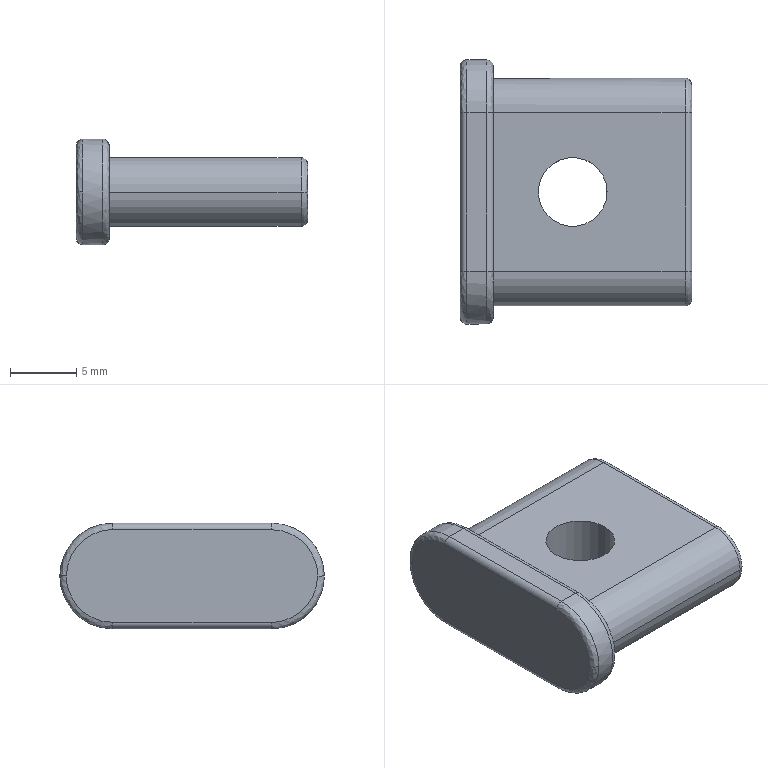Part | SolidWorks | features BaseBody 1 | 1 solid | 31 faces | box 17.5 x 20 x 8 mm | volume 1504 mm3 | cylinder 14 | spline 10 | plane 7 | commonest cylinder face diameters 1 x6 5.2 x5 8 x3
STEP:
#1=CARTESIAN_POINT('',(-91538.135,-120061.55,4564.099));
#2=VERTEX_POINT('',#1);
#3=CARTESIAN_POINT('',(-91538.135,-120058.95,4566.699));
#4=VERTEX_POINT('',#3);
#5=CARTESIAN_POINT('',(-91538.135,-120058.95,4564.099));
#6=DIRECTION('',(-1.,0.000000008,0.));
#7=DIRECTION('',(-0.000000008,-1.,0.));
#8=AXIS2_PLACEMENT_3D('',#5,#6,#7);
#9=CIRCLE('',#8,2.6);
#10=EDGE_CURVE('',#2,#4,#9,.T.);
#11=ORIENTED_EDGE('',*,*,#10,.F.);
#12=CARTESIAN_POINT('',(-91537.635,-120061.05,4564.099));
#13=VERTEX_POINT('',#12);
#14=CARTESIAN_POINT('',(-91538.135,-120061.05,4564.099));
#15=DIRECTION('',(0.,0.,1.));
#16=DIRECTION('',(-0.000000008,-1.,0.));
#17=AXIS2_PLACEMENT_3D('',#14,#15,#16);
#18=CIRCLE('',#17,0.5);
#19=EDGE_CURVE('',#2,#13,#18,.T.);
#20=ORIENTED_EDGE('',*,*,#19,.T.);
#21=CARTESIAN_POINT('',(-91537.635,-120058.95,4566.199));
#22=VERTEX_POINT('',#21);
#23=CARTESIAN_POINT('',(-91537.635,-120061.05,4564.099));
#24=CARTESIAN_POINT('',(-91537.635,-120061.05,4565.329));
#25=CARTESIAN_POINT('',(-91537.635,-120060.18,4566.199));
#26=CARTESIAN_POINT('',(-91537.635,-120058.95,4566.199));
#27=(BOUNDED_CURVE()B_SPLINE_CURVE(3,(#23,#24,#25,#26),.UNSPECIFIED.,.F.,.T.)B_SPLINE_CURVE_WITH_KNOTS((4,4),(0.,1.),.UNSPECIFIED.)CURVE()GEOMETRIC_REPRESENTATION_ITEM()RATIONAL_B_SPLINE_CURVE((1.,0.8047,0.8047,1.))REPRESENTATION_ITEM(''));
#28=EDGE_CURVE('',#13,#22,#27,.T.);
#29=ORIENTED_EDGE('',*,*,#28,.T.);
#30=CARTESIAN_POINT('',(-91538.135,-120058.95,4566.199));
#31=DIRECTION('',(-0.000000008,-1.,0.));
#32=DIRECTION('',(0.,0.,1.));
#33=AXIS2_PLACEMENT_3D('',#30,#31,#32);
#34=CIRCLE('',#33,0.5);
#35=EDGE_CURVE('',#22,#4,#34,.T.);
#36=ORIENTED_EDGE('',*,*,#35,.T.);
#37=EDGE_LOOP('',(#11,#20,#29,#36));
#38=FACE_OUTER_BOUND('',#37,.T.);
#39=CARTESIAN_POINT('',(-91538.135,-120061.55,4564.099));
#40=CARTESIAN_POINT('',(-91538.135,-120061.55,4565.633));
#41=CARTESIAN_POINT('',(-91538.135,-120060.46,4566.713));
#42=CARTESIAN_POINT('',(-91538.135,-120058.925,4566.699));
#43=CARTESIAN_POINT('',(-91537.842,-120061.55,4564.099));
#44=CARTESIAN_POINT('',(-91537.842,-120061.55,4565.633));
#45=CARTESIAN_POINT('',(-91537.842,-120060.46,4566.713));
#46=CARTESIAN_POINT('',(-91537.842,-120058.925,4566.699));
#47=CARTESIAN_POINT('',(-91537.635,-120061.343,4564.099));
#48=CARTESIAN_POINT('',(-91537.635,-120061.343,4565.511));
#49=CARTESIAN_POINT('',(-91537.635,-120060.34,4566.505));
#50=CARTESIAN_POINT('',(-91537.635,-120058.927,4566.492));
#51=CARTESIAN_POINT('',(-91537.635,-120061.05,4564.099));
#52=CARTESIAN_POINT('',(-91537.635,-120061.05,4565.338));
#53=CARTESIAN_POINT('',(-91537.635,-120060.17,4566.211));
#54=CARTESIAN_POINT('',(-91537.635,-120058.93,4566.199));
#55=(BOUNDED_SURFACE()B_SPLINE_SURFACE(3,3,((#39,#40,#41,#42),(#43,#44,#45,#46),(#47,#48,#49,#50),(#51,#52,#53,#54)),.UNSPECIFIED.,.F.,.F.,.F.)B_SPLINE_SURFACE_WITH_KNOTS((4,4),(4,4),(0.,1.),(0.,1.),.UNSPECIFIED.)GEOMETRIC_REPRESENTATION_ITEM()RATIONAL_B_SPLINE_SURFACE(((1.,0.8025,0.8025,1.),(0.8047,0.6458,0.6458,0.8047),(0.8047,0.6458,0.6458,0.8047),(1.,0.8025,0.8025,1.)))REPRESENTATION_ITEM('')SURFACE());
#56=ADVANCED_FACE('',(#38),#55,.T.);
#57=CARTESIAN_POINT('',(-91555.135,-120058.95,4567.599));
#58=VERTEX_POINT('',#57);
#59=CARTESIAN_POINT('',(-91555.135,-120062.45,4564.099));
#60=VERTEX_POINT('',#59);
#61=CARTESIAN_POINT('',(-91555.135,-120058.95,4567.599));
#62=CARTESIAN_POINT('',(-91555.135,-120061.,4567.599));
#63=CARTESIAN_POINT('',(-91555.135,-120062.45,4566.149));
#64=CARTESIAN_POINT('',(-91555.135,-120062.45,4564.099));
#65=(BOUNDED_CURVE()B_SPLINE_CURVE(3,(#61,#62,#63,#64),.UNSPECIFIED.,.F.,.T.)B_SPLINE_CURVE_WITH_KNOTS((4,4),(0.,1.),.UNSPECIFIED.)CURVE()GEOMETRIC_REPRESENTATION_ITEM()RATIONAL_B_SPLINE_CURVE((1.,0.8047,0.8047,1.))REPRESENTATION_ITEM(''));
#66=EDGE_CURVE('',#58,#60,#65,.T.);
#67=ORIENTED_EDGE('',*,*,#66,.T.);
#68=CARTESIAN_POINT('',(-91554.635,-120062.95,4564.099));
#69=VERTEX_POINT('',#68);
#70=CARTESIAN_POINT('',(-91554.635,-120062.45,4564.099));
#71=DIRECTION('',(0.,0.,1.));
#72=DIRECTION('',(-0.000000008,-1.,0.));
#73=AXIS2_PLACEMENT_3D('',#70,#71,#72);
#74=CIRCLE('',#73,0.5);
#75=EDGE_CURVE('',#60,#69,#74,.T.);
#76=ORIENTED_EDGE('',*,*,#75,.T.);
#77=CARTESIAN_POINT('',(-91554.635,-120058.95,4568.099));
#78=VERTEX_POINT('',#77);
#79=CARTESIAN_POINT('',(-91554.635,-120058.95,4564.099));
#80=DIRECTION('',(1.,-0.000000008,0.));
#81=DIRECTION('',(0.000000008,1.,0.));
#82=AXIS2_PLACEMENT_3D('',#79,#80,#81);
#83=CIRCLE('',#82,4.);
#84=EDGE_CURVE('',#78,#69,#83,.T.);
#85=ORIENTED_EDGE('',*,*,#84,.F.);
#86=CARTESIAN_POINT('',(-91554.635,-120058.95,4567.599));
#87=DIRECTION('',(0.000000008,1.,0.));
#88=DIRECTION('',(-1.,0.000000008,0.));
#89=AXIS2_PLACEMENT_3D('',#86,#87,#88);
#90=CIRCLE('',#89,0.5);
#91=EDGE_CURVE('',#58,#78,#90,.T.);
#92=ORIENTED_EDGE('',*,*,#91,.F.);
#93=EDGE_LOOP('',(#67,#76,#85,#92));
#94=FACE_OUTER_BOUND('',#93,.T.);
#95=CARTESIAN_POINT('',(-91555.135,-120062.45,4564.099));
#96=CARTESIAN_POINT('',(-91555.135,-120062.45,4566.149));
#97=CARTESIAN_POINT('',(-91555.135,-120061.,4567.599));
#98=CARTESIAN_POINT('',(-91555.135,-120058.95,4567.599));
#99=CARTESIAN_POINT('',(-91555.135,-120062.743,4564.099));
#100=CARTESIAN_POINT('',(-91555.135,-120062.743,4566.321));
#101=CARTESIAN_POINT('',(-91555.135,-120061.172,4567.892));
#102=CARTESIAN_POINT('',(-91555.135,-120058.95,4567.892));
#103=CARTESIAN_POINT('',(-91554.928,-120062.95,4564.099));
#104=CARTESIAN_POINT('',(-91554.928,-120062.95,4566.442));
#105=CARTESIAN_POINT('',(-91554.928,-120061.293,4568.099));
#106=CARTESIAN_POINT('',(-91554.928,-120058.95,4568.099));
#107=CARTESIAN_POINT('',(-91554.635,-120062.95,4564.099));
#108=CARTESIAN_POINT('',(-91554.635,-120062.95,4566.442));
#109=CARTESIAN_POINT('',(-91554.635,-120061.293,4568.099));
#110=CARTESIAN_POINT('',(-91554.635,-120058.95,4568.099));
#111=(BOUNDED_SURFACE()B_SPLINE_SURFACE(3,3,((#95,#96,#97,#98),(#99,#100,#101,#102),(#103,#104,#105,#106),(#107,#108,#109,#110)),.UNSPECIFIED.,.F.,.F.,.T.)B_SPLINE_SURFACE_WITH_KNOTS((4,4),(4,4),(0.,1.),(0.,1.),.UNSPECIFIED.)GEOMETRIC_REPRESENTATION_ITEM()RATIONAL_B_SPLINE_SURFACE(((1.,0.8047,0.8047,1.),(0.8047,0.6476,0.6476,0.8047),(0.8047,0.6476,0.6476,0.8047),(1.,0.8047,0.8047,1.)))REPRESENTATION_ITEM('')SURFACE());
#112=ADVANCED_FACE('',(#94),#111,.T.);
#113=CARTESIAN_POINT('',(-91538.135,-120058.95,4561.499));
#114=VERTEX_POINT('',#113);
#115=CARTESIAN_POINT('',(-91538.135,-120058.95,4564.099));
#116=DIRECTION('',(-1.,0.000000008,0.));
#117=DIRECTION('',(-0.000000008,-1.,0.));
#118=AXIS2_PLACEMENT_3D('',#115,#116,#117);
#119=CIRCLE('',#118,2.6);
#120=EDGE_CURVE('',#114,#2,#119,.T.);
#121=ORIENTED_EDGE('',*,*,#120,.T.);
#122=CARTESIAN_POINT('',(-91552.635,-120061.55,4564.099));
#123=VERTEX_POINT('',#122);
#124=CARTESIAN_POINT('',(-91519.666,-120061.55,4564.099));
#125=DIRECTION('',(-1.,0.000000008,0.));
#126=VECTOR('',#125,1000.);
#127=LINE('',#124,#126);
#128=EDGE_CURVE('',#2,#123,#127,.T.);
#129=ORIENTED_EDGE('',*,*,#128,.T.);
#130=CARTESIAN_POINT('',(-91552.635,-120058.95,4561.499));
#131=VERTEX_POINT('',#130);
#132=CARTESIAN_POINT('',(-91552.635,-120058.95,4564.099));
#133=DIRECTION('',(1.,-0.000000008,0.));
#134=DIRECTION('',(-0.000000008,-1.,0.));
#135=AXIS2_PLACEMENT_3D('',#132,#133,#134);
#136=CIRCLE('',#135,2.6);
#137=EDGE_CURVE('',#123,#131,#136,.T.);
#138=ORIENTED_EDGE('',*,*,#137,.T.);
#139=CARTESIAN_POINT('',(-91537.635,-120058.95,4561.499));
#140=DIRECTION('',(-1.,0.,0.));
#141=VECTOR('',#140,1000.);
#142=LINE('',#139,#141);
#143=EDGE_CURVE('',#114,#131,#142,.T.);
#144=ORIENTED_EDGE('',*,*,#143,.F.);
#145=EDGE_LOOP('',(#121,#129,#138,#144));
#146=FACE_OUTER_BOUND('',#145,.T.);
#147=CARTESIAN_POINT('',(-91519.666,-120058.95,4564.099));
#148=DIRECTION('',(-1.,0.000000008,0.));
#149=DIRECTION('',(-0.000000008,-1.,0.));
#150=AXIS2_PLACEMENT_3D('',#147,#148,#149);
#151=CYLINDRICAL_SURFACE('',#150,2.6);
#152=ADVANCED_FACE('',(#146),#151,.T.);
#153=CARTESIAN_POINT('',(-91544.035,-120052.95,4566.699));
#154=VERTEX_POINT('',#153);
#155=CARTESIAN_POINT('',(-91549.235,-120052.95,4566.699));
#156=VERTEX_POINT('',#155);
#157=CARTESIAN_POINT('',(-91546.635,-120052.95,4566.699));
#158=DIRECTION('',(0.,0.,-1.));
#159=DIRECTION('',(-1.,0.,0.));
#160=AXIS2_PLACEMENT_3D('',#157,#158,#159);
#161=CIRCLE('',#160,2.6);
#162=EDGE_CURVE('',#154,#156,#161,.T.);
#163=ORIENTED_EDGE('',*,*,#162,.F.);
#164=CARTESIAN_POINT('',(-91544.035,-120052.95,4561.499));
#165=VERTEX_POINT('',#164);
#166=CARTESIAN_POINT('',(-91544.035,-120052.95,4571.499));
#167=DIRECTION('',(0.,0.,-1.));
#168=VECTOR('',#167,1000.);
#169=LINE('',#166,#168);
#170=EDGE_CURVE('',#154,#165,#169,.T.);
#171=ORIENTED_EDGE('',*,*,#170,.T.);
#172=CARTESIAN_POINT('',(-91549.235,-120052.95,4561.499));
#173=VERTEX_POINT('',#172);
#174=CARTESIAN_POINT('',(-91546.635,-120052.95,4561.499));
#175=DIRECTION('',(0.,0.,1.));
#176=DIRECTION('',(-1.,0.,0.));
#177=AXIS2_PLACEMENT_3D('',#174,#175,#176);
#178=CIRCLE('',#177,2.6);
#179=EDGE_CURVE('',#173,#165,#178,.T.);
#180=ORIENTED_EDGE('',*,*,#179,.F.);
#181=CARTESIAN_POINT('',(-91549.235,-120052.95,4571.499));
#182=DIRECTION('',(0.,0.,-1.));
#183=VECTOR('',#182,1000.);
#184=LINE('',#181,#183);
#185=EDGE_CURVE('',#156,#173,#184,.T.);
#186=ORIENTED_EDGE('',*,*,#185,.F.);
#187=EDGE_LOOP('',(#163,#171,#180,#186));
#188=FACE_OUTER_BOUND('',#187,.T.);
#189=CARTESIAN_POINT('',(-91546.635,-120052.95,4571.499));
#190=DIRECTION('',(0.,0.,-1.));
#191=DIRECTION('',(-1.,0.,0.));
#192=AXIS2_PLACEMENT_3D('',#189,#190,#191);
#193=CYLINDRICAL_SURFACE('',#192,2.6);
#194=ADVANCED_FACE('',(#188),#193,.F.);
#195=CARTESIAN_POINT('',(-91554.635,-120046.95,4560.099));
#196=VERTEX_POINT('',#195);
#197=CARTESIAN_POINT('',(-91554.635,-120042.95,4564.099));
#198=VERTEX_POINT('',#197);
#199=CARTESIAN_POINT('',(-91554.635,-120046.95,4564.099));
#200=DIRECTION('',(1.,-0.000000008,0.));
#201=DIRECTION('',(0.000000008,1.,0.));
#202=AXIS2_PLACEMENT_3D('',#199,#200,#201);
#203=CIRCLE('',#202,4.);
#204=EDGE_CURVE('',#196,#198,#203,.T.);
#205=ORIENTED_EDGE('',*,*,#204,.T.);
#206=CARTESIAN_POINT('',(-91553.135,-120042.95,4564.099));
#207=VERTEX_POINT('',#206);
#208=CARTESIAN_POINT('',(-91576.676,-120042.95,4564.099));
#209=DIRECTION('',(1.,-0.000000008,0.));
#210=VECTOR('',#209,1000.);
#211=LINE('',#208,#210);
#212=EDGE_CURVE('',#198,#207,#211,.T.);
#213=ORIENTED_EDGE('',*,*,#212,.T.);
#214=CARTESIAN_POINT('',(-91553.135,-120046.95,4560.099));
#215=VERTEX_POINT('',#214);
#216=CARTESIAN_POINT('',(-91553.135,-120046.95,4564.099));
#217=DIRECTION('',(1.,-0.000000008,0.));
#218=DIRECTION('',(0.000000008,1.,0.));
#219=AXIS2_PLACEMENT_3D('',#216,#217,#218);
#220=CIRCLE('',#219,4.);
#221=EDGE_CURVE('',#215,#207,#220,.T.);
#222=ORIENTED_EDGE('',*,*,#221,.F.);
#223=CARTESIAN_POINT('',(-91576.676,-120046.95,4560.099));
#224=DIRECTION('',(-1.,0.000000008,0.));
#225=VECTOR('',#224,1000.);
#226=LINE('',#223,#225);
#227=EDGE_CURVE('',#215,#196,#226,.T.);
#228=ORIENTED_EDGE('',*,*,#227,.T.);
#229=EDGE_LOOP('',(#205,#213,#222,#228));
#230=FACE_OUTER_BOUND('',#229,.T.);
#231=CARTESIAN_POINT('',(-91576.676,-120046.95,4564.099));
#232=DIRECTION('',(1.,-0.000000008,0.));
#233=DIRECTION('',(0.000000008,1.,0.));
#234=AXIS2_PLACEMENT_3D('',#231,#232,#233);
#235=CYLINDRICAL_SURFACE('',#234,4.);
#236=ADVANCED_FACE('',(#230),#235,.T.);
#237=ORIENTED_EDGE('',*,*,#143,.T.);
#238=CARTESIAN_POINT('',(-91552.635,-120046.95,4561.499));
#239=VERTEX_POINT('',#238);
#240=CARTESIAN_POINT('',(-91552.635,-120048.95,4561.499));
#241=DIRECTION('',(0.,1.,0.));
#242=VECTOR('',#241,1000.);
#243=LINE('',#240,#242);
#244=EDGE_CURVE('',#131,#239,#243,.T.);
#245=ORIENTED_EDGE('',*,*,#244,.T.);
#246=CARTESIAN_POINT('',(-91538.135,-120046.95,4561.499));
#247=VERTEX_POINT('',#246);
#248=CARTESIAN_POINT('',(-91537.635,-120046.95,4561.499));
#249=DIRECTION('',(1.,0.,0.));
#250=VECTOR('',#249,1000.);
#251=LINE('',#248,#250);
#252=EDGE_CURVE('',#239,#247,#251,.T.);
#253=ORIENTED_EDGE('',*,*,#252,.T.);
#254=CARTESIAN_POINT('',(-91538.135,-120048.95,4561.499));
#255=DIRECTION('',(0.,-1.,0.));
#256=VECTOR('',#255,1000.);
#257=LINE('',#254,#256);
#258=EDGE_CURVE('',#247,#114,#257,.T.);
#259=ORIENTED_EDGE('',*,*,#258,.T.);
#260=EDGE_LOOP('',(#237,#245,#253,#259));
#261=FACE_OUTER_BOUND('',#260,.T.);
#262=ORIENTED_EDGE('',*,*,#179,.T.);
#263=CARTESIAN_POINT('',(-91546.635,-120052.95,4561.499));
#264=DIRECTION('',(0.,0.,1.));
#265=DIRECTION('',(-1.,0.,0.));
#266=AXIS2_PLACEMENT_3D('',#263,#264,#265);
#267=CIRCLE('',#266,2.6);
#268=EDGE_CURVE('',#165,#173,#267,.T.);
#269=ORIENTED_EDGE('',*,*,#268,.T.);
#270=EDGE_LOOP('',(#262,#269));
#271=FACE_BOUND('',#270,.T.);
#272=CARTESIAN_POINT('',(-91537.635,-120048.95,4561.499));
#273=DIRECTION('',(0.,0.,-1.));
#274=DIRECTION('',(-1.,0.,0.));
#275=AXIS2_PLACEMENT_3D('',#272,#273,#274);
#276=PLANE('',#275);
#277=ADVANCED_FACE('',(#261,#271),#276,.T.);
#278=CARTESIAN_POINT('',(-91552.635,-120058.95,4566.699));
#279=VERTEX_POINT('',#278);
#280=CARTESIAN_POINT('',(-91552.635,-120058.95,4564.099));
#281=DIRECTION('',(1.,-0.000000008,0.));
#282=DIRECTION('',(-0.000000008,-1.,0.));
#283=AXIS2_PLACEMENT_3D('',#280,#281,#282);
#284=CIRCLE('',#283,2.6);
#285=EDGE_CURVE('',#279,#123,#284,.T.);
#286=ORIENTED_EDGE('',*,*,#285,.F.);
#287=CARTESIAN_POINT('',(-91552.635,-120046.95,4566.699));
#288=VERTEX_POINT('',#287);
#289=CARTESIAN_POINT('',(-91552.635,-120056.95,4566.699));
#290=DIRECTION('',(-0.000000008,-1.,0.));
#291=VECTOR('',#290,1000.);
#292=LINE('',#289,#291);
#293=EDGE_CURVE('',#288,#279,#292,.T.);
#294=ORIENTED_EDGE('',*,*,#293,.F.);
#295=CARTESIAN_POINT('',(-91552.635,-120046.95,4564.099));
#296=DIRECTION('',(1.,-0.000000008,0.));
#297=DIRECTION('',(-0.000000008,-1.,0.));
#298=AXIS2_PLACEMENT_3D('',#295,#296,#297);
#299=CIRCLE('',#298,2.6);
#300=EDGE_CURVE('',#239,#288,#299,.T.);
#301=ORIENTED_EDGE('',*,*,#300,.F.);
#302=ORIENTED_EDGE('',*,*,#244,.F.);
#303=ORIENTED_EDGE('',*,*,#137,.F.);
#304=EDGE_LOOP('',(#286,#294,#301,#302,#303));
#305=FACE_BOUND('',#304,.T.);
#306=CARTESIAN_POINT('',(-91552.635,-120058.95,4567.599));
#307=VERTEX_POINT('',#306);
#308=CARTESIAN_POINT('',(-91552.635,-120046.95,4567.599));
#309=VERTEX_POINT('',#308);
#310=CARTESIAN_POINT('',(-91552.635,-120056.95,4567.599));
#311=DIRECTION('',(0.000000008,1.,0.));
#312=VECTOR('',#311,1000.);
#313=LINE('',#310,#312);
#314=EDGE_CURVE('',#307,#309,#313,.T.);
#315=ORIENTED_EDGE('',*,*,#314,.F.);
#316=CARTESIAN_POINT('',(-91552.635,-120058.95,4560.599));
#317=VERTEX_POINT('',#316);
#318=CARTESIAN_POINT('',(-91552.635,-120058.95,4560.599));
#319=CARTESIAN_POINT('',(-91552.635,-120065.95,4560.599));
#320=CARTESIAN_POINT('',(-91552.635,-120065.95,4567.599));
#321=CARTESIAN_POINT('',(-91552.635,-120058.95,4567.599));
#322=(BOUNDED_CURVE()B_SPLINE_CURVE(3,(#318,#319,#320,#321),.UNSPECIFIED.,.F.,.F.)B_SPLINE_CURVE_WITH_KNOTS((4,4),(0.,1.),.UNSPECIFIED.)CURVE()GEOMETRIC_REPRESENTATION_ITEM()RATIONAL_B_SPLINE_CURVE((1.,0.3333,0.3333,1.))REPRESENTATION_ITEM(''));
#323=EDGE_CURVE('',#317,#307,#322,.T.);
#324=ORIENTED_EDGE('',*,*,#323,.F.);
#325=CARTESIAN_POINT('',(-91552.635,-120046.95,4560.599));
#326=VERTEX_POINT('',#325);
#327=CARTESIAN_POINT('',(-91552.635,-120056.95,4560.599));
#328=DIRECTION('',(-0.000000008,-1.,0.));
#329=VECTOR('',#328,1000.);
#330=LINE('',#327,#329);
#331=EDGE_CURVE('',#326,#317,#330,.T.);
#332=ORIENTED_EDGE('',*,*,#331,.F.);
#333=CARTESIAN_POINT('',(-91552.635,-120046.95,4567.599));
#334=CARTESIAN_POINT('',(-91552.635,-120039.95,4567.599));
#335=CARTESIAN_POINT('',(-91552.635,-120039.95,4560.599));
#336=CARTESIAN_POINT('',(-91552.635,-120046.95,4560.599));
#337=(BOUNDED_CURVE()B_SPLINE_CURVE(3,(#333,#334,#335,#336),.UNSPECIFIED.,.F.,.F.)B_SPLINE_CURVE_WITH_KNOTS((4,4),(0.,1.),.UNSPECIFIED.)CURVE()GEOMETRIC_REPRESENTATION_ITEM()RATIONAL_B_SPLINE_CURVE((1.,0.3333,0.3333,1.))REPRESENTATION_ITEM(''));
#338=EDGE_CURVE('',#309,#326,#337,.T.);
#339=ORIENTED_EDGE('',*,*,#338,.F.);
#340=EDGE_LOOP('',(#315,#324,#332,#339));
#341=FACE_OUTER_BOUND('',#340,.T.);
#342=CARTESIAN_POINT('',(-91552.635,-120056.95,4564.099));
#343=DIRECTION('',(-1.,0.000000008,0.));
#344=DIRECTION('',(-0.000000008,-1.,0.));
#345=AXIS2_PLACEMENT_3D('',#342,#343,#344);
#346=PLANE('',#345);
#347=ADVANCED_FACE('',(#305,#341),#346,.F.);
#348=ORIENTED_EDGE('',*,*,#128,.F.);
#349=ORIENTED_EDGE('',*,*,#10,.T.);
#350=CARTESIAN_POINT('',(-91519.666,-120058.95,4566.699));
#351=DIRECTION('',(-1.,0.000000008,0.));
#352=VECTOR('',#351,1000.);
#353=LINE('',#350,#352);
#354=EDGE_CURVE('',#4,#279,#353,.T.);
#355=ORIENTED_EDGE('',*,*,#354,.T.);
#356=ORIENTED_EDGE('',*,*,#285,.T.);
#357=EDGE_LOOP('',(#348,#349,#355,#356));
#358=FACE_OUTER_BOUND('',#357,.T.);
#359=CARTESIAN_POINT('',(-91519.666,-120058.95,4564.099));
#360=DIRECTION('',(-1.,0.000000008,0.));
#361=DIRECTION('',(-0.000000008,-1.,0.));
#362=AXIS2_PLACEMENT_3D('',#359,#360,#361);
#363=CYLINDRICAL_SURFACE('',#362,2.6);
#364=ADVANCED_FACE('',(#358),#363,.T.);
#365=CARTESIAN_POINT('',(-91537.635,-120058.95,4561.999));
#366=VERTEX_POINT('',#365);
#367=CARTESIAN_POINT('',(-91538.135,-120058.95,4561.999));
#368=DIRECTION('',(0.000000008,1.,0.));
#369=DIRECTION('',(-1.,0.000000008,0.));
#370=AXIS2_PLACEMENT_3D('',#367,#368,#369);
#371=CIRCLE('',#370,0.5);
#372=EDGE_CURVE('',#366,#114,#371,.T.);
#373=ORIENTED_EDGE('',*,*,#372,.T.);
#374=ORIENTED_EDGE('',*,*,#258,.F.);
#375=CARTESIAN_POINT('',(-91537.635,-120046.95,4561.999));
#376=VERTEX_POINT('',#375);
#377=CARTESIAN_POINT('',(-91538.135,-120046.95,4561.999));
#378=DIRECTION('',(0.000000008,1.,0.));
#379=DIRECTION('',(-1.,0.000000008,0.));
#380=AXIS2_PLACEMENT_3D('',#377,#378,#379);
#381=CIRCLE('',#380,0.5);
#382=EDGE_CURVE('',#376,#247,#381,.T.);
#383=ORIENTED_EDGE('',*,*,#382,.F.);
#384=CARTESIAN_POINT('',(-91537.635,-120048.95,4561.999));
#385=DIRECTION('',(-0.000000008,-1.,0.));
#386=VECTOR('',#385,1000.);
#387=LINE('',#384,#386);
#388=EDGE_CURVE('',#376,#366,#387,.T.);
#389=ORIENTED_EDGE('',*,*,#388,.T.);
#390=EDGE_LOOP('',(#373,#374,#383,#389));
#391=FACE_OUTER_BOUND('',#390,.T.);
#392=CARTESIAN_POINT('',(-91538.135,-120048.95,4561.999));
#393=DIRECTION('',(0.000000008,1.,0.));
#394=DIRECTION('',(-1.,0.000000008,0.));
#395=AXIS2_PLACEMENT_3D('',#392,#393,#394);
#396=CYLINDRICAL_SURFACE('',#395,0.5);
#397=ADVANCED_FACE('',(#391),#396,.T.);
#398=CARTESIAN_POINT('',(-91538.135,-120046.95,4566.699));
#399=VERTEX_POINT('',#398);
#400=CARTESIAN_POINT('',(-91519.666,-120046.95,4566.699));
#401=DIRECTION('',(1.,-0.000000008,0.));
#402=VECTOR('',#401,1000.);
#403=LINE('',#400,#402);
#404=EDGE_CURVE('',#288,#399,#403,.T.);
#405=ORIENTED_EDGE('',*,*,#404,.T.);
#406=CARTESIAN_POINT('',(-91538.135,-120044.35,4564.099));
#407=VERTEX_POINT('',#406);
#408=CARTESIAN_POINT('',(-91538.135,-120046.95,4564.099));
#409=DIRECTION('',(-1.,0.000000008,0.));
#410=DIRECTION('',(-0.000000008,-1.,0.));
#411=AXIS2_PLACEMENT_3D('',#408,#409,#410);
#412=CIRCLE('',#411,2.6);
#413=EDGE_CURVE('',#399,#407,#412,.T.);
#414=ORIENTED_EDGE('',*,*,#413,.T.);
#415=CARTESIAN_POINT('',(-91538.135,-120046.95,4564.099));
#416=DIRECTION('',(-1.,0.000000008,0.));
#417=DIRECTION('',(-0.000000008,-1.,0.));
#418=AXIS2_PLACEMENT_3D('',#415,#416,#417);
#419=CIRCLE('',#418,2.6);
#420=EDGE_CURVE('',#407,#247,#419,.T.);
#421=ORIENTED_EDGE('',*,*,#420,.T.);
#422=ORIENTED_EDGE('',*,*,#252,.F.);
#423=ORIENTED_EDGE('',*,*,#300,.T.);
#424=EDGE_LOOP('',(#405,#414,#421,#422,#423));
#425=FACE_OUTER_BOUND('',#424,.T.);
#426=CARTESIAN_POINT('',(-91519.666,-120046.95,4564.099));
#427=DIRECTION('',(-1.,0.000000008,0.));
#428=DIRECTION('',(-0.000000008,-1.,0.));
#429=AXIS2_PLACEMENT_3D('',#426,#427,#428);
#430=CYLINDRICAL_SURFACE('',#429,2.6);
#431=ADVANCED_FACE('',(#425),#430,.T.);
#432=ORIENTED_EDGE('',*,*,#170,.F.);
#433=CARTESIAN_POINT('',(-91546.635,-120052.95,4566.699));
#434=DIRECTION('',(0.,0.,-1.));
#435=DIRECTION('',(-1.,0.,0.));
#436=AXIS2_PLACEMENT_3D('',#433,#434,#435);
#437=CIRCLE('',#436,2.6);
#438=EDGE_CURVE('',#156,#154,#437,.T.);
#439=ORIENTED_EDGE('',*,*,#438,.F.);
#440=ORIENTED_EDGE('',*,*,#185,.T.);
#441=ORIENTED_EDGE('',*,*,#268,.F.);
#442=EDGE_LOOP('',(#432,#439,#440,#441));
#443=FACE_OUTER_BOUND('',#442,.T.);
#444=CARTESIAN_POINT('',(-91546.635,-120052.95,4571.499));
#445=DIRECTION('',(0.,0.,-1.));
#446=DIRECTION('',(-1.,0.,0.));
#447=AXIS2_PLACEMENT_3D('',#444,#445,#446);
#448=CYLINDRICAL_SURFACE('',#447,2.6);
#449=ADVANCED_FACE('',(#443),#448,.F.);
#450=ORIENTED_EDGE('',*,*,#404,.F.);
#451=ORIENTED_EDGE('',*,*,#293,.T.);
#452=ORIENTED_EDGE('',*,*,#354,.F.);
#453=CARTESIAN_POINT('',(-91538.135,-120056.95,4566.699));
#454=DIRECTION('',(0.,1.,0.));
#455=VECTOR('',#454,1000.);
#456=LINE('',#453,#455);
#457=EDGE_CURVE('',#4,#399,#456,.T.);
#458=ORIENTED_EDGE('',*,*,#457,.T.);
#459=EDGE_LOOP('',(#450,#451,#452,#458));
#460=FACE_OUTER_BOUND('',#459,.T.);
#461=ORIENTED_EDGE('',*,*,#438,.T.);
#462=ORIENTED_EDGE('',*,*,#162,.T.);
#463=EDGE_LOOP('',(#461,#462));
#464=FACE_BOUND('',#463,.T.);
#465=CARTESIAN_POINT('',(-91537.635,-120056.95,4566.699));
#466=DIRECTION('',(0.,0.,1.));
#467=DIRECTION('',(1.,0.,0.));
#468=AXIS2_PLACEMENT_3D('',#465,#466,#467);
#469=PLANE('',#468);
#470=ADVANCED_FACE('',(#460,#464),#469,.T.);
#471=ORIENTED_EDGE('',*,*,#221,.T.);
#472=CARTESIAN_POINT('',(-91553.135,-120046.95,4568.099));
#473=VERTEX_POINT('',#472);
#474=CARTESIAN_POINT('',(-91553.135,-120046.95,4564.099));
#475=DIRECTION('',(1.,-0.000000008,0.));
#476=DIRECTION('',(0.000000008,1.,0.));
#477=AXIS2_PLACEMENT_3D('',#474,#475,#476);
#478=CIRCLE('',#477,4.);
#479=EDGE_CURVE('',#207,#473,#478,.T.);
#480=ORIENTED_EDGE('',*,*,#479,.T.);
#481=CARTESIAN_POINT('',(-91553.135,-120046.95,4567.599));
#482=DIRECTION('',(0.000000008,1.,0.));
#483=DIRECTION('',(-1.,0.000000008,0.));
#484=AXIS2_PLACEMENT_3D('',#481,#482,#483);
#485=CIRCLE('',#484,0.5);
#486=EDGE_CURVE('',#473,#309,#485,.T.);
#487=ORIENTED_EDGE('',*,*,#486,.T.);
#488=ORIENTED_EDGE('',*,*,#338,.T.);
#489=CARTESIAN_POINT('',(-91553.135,-120046.95,4560.599));
#490=DIRECTION('',(0.000000008,1.,0.));
#491=DIRECTION('',(-1.,0.000000008,0.));
#492=AXIS2_PLACEMENT_3D('',#489,#490,#491);
#493=CIRCLE('',#492,0.5);
#494=EDGE_CURVE('',#326,#215,#493,.T.);
#495=ORIENTED_EDGE('',*,*,#494,.T.);
#496=EDGE_LOOP('',(#471,#480,#487,#488,#495));
#497=FACE_OUTER_BOUND('',#496,.T.);
#498=CARTESIAN_POINT('',(-91553.135,-120046.95,4568.099));
#499=CARTESIAN_POINT('',(-91553.135,-120038.95,4568.099));
#500=CARTESIAN_POINT('',(-91553.135,-120038.95,4560.099));
#501=CARTESIAN_POINT('',(-91553.135,-120046.95,4560.099));
#502=CARTESIAN_POINT('',(-91552.842,-120046.95,4568.099));
#503=CARTESIAN_POINT('',(-91552.842,-120038.95,4568.099));
#504=CARTESIAN_POINT('',(-91552.842,-120038.95,4560.099));
#505=CARTESIAN_POINT('',(-91552.842,-120046.95,4560.099));
#506=CARTESIAN_POINT('',(-91552.635,-120046.95,4567.892));
#507=CARTESIAN_POINT('',(-91552.635,-120039.364,4567.892));
#508=CARTESIAN_POINT('',(-91552.635,-120039.364,4560.306));
#509=CARTESIAN_POINT('',(-91552.635,-120046.95,4560.306));
#510=CARTESIAN_POINT('',(-91552.635,-120046.95,4567.599));
#511=CARTESIAN_POINT('',(-91552.635,-120039.95,4567.599));
#512=CARTESIAN_POINT('',(-91552.635,-120039.95,4560.599));
#513=CARTESIAN_POINT('',(-91552.635,-120046.95,4560.599));
#514=(BOUNDED_SURFACE()B_SPLINE_SURFACE(3,3,((#498,#499,#500,#501),(#502,#503,#504,#505),(#506,#507,#508,#509),(#510,#511,#512,#513)),.UNSPECIFIED.,.F.,.F.,.T.)B_SPLINE_SURFACE_WITH_KNOTS((4,4),(4,4),(0.,1.),(0.,1.),.UNSPECIFIED.)GEOMETRIC_REPRESENTATION_ITEM()RATIONAL_B_SPLINE_SURFACE(((1.,0.3333,0.3333,1.),(0.8047,0.2682,0.2682,0.8047),(0.8047,0.2682,0.2682,0.8047),(1.,0.3333,0.3333,1.)))REPRESENTATION_ITEM('')SURFACE());
#515=ADVANCED_FACE('',(#497),#514,.T.);
#516=CARTESIAN_POINT('',(-91553.135,-120058.95,4568.099));
#517=VERTEX_POINT('',#516);
#518=CARTESIAN_POINT('',(-91553.135,-120058.95,4567.599));
#519=DIRECTION('',(0.000000008,1.,0.));
#520=DIRECTION('',(1.,-0.000000008,0.));
#521=AXIS2_PLACEMENT_3D('',#518,#519,#520);
#522=CIRCLE('',#521,0.5);
#523=EDGE_CURVE('',#517,#307,#522,.T.);
#524=ORIENTED_EDGE('',*,*,#523,.T.);
#525=ORIENTED_EDGE('',*,*,#314,.T.);
#526=ORIENTED_EDGE('',*,*,#486,.F.);
#527=CARTESIAN_POINT('',(-91553.135,-120056.95,4568.099));
#528=DIRECTION('',(-0.000000008,-1.,0.));
#529=VECTOR('',#528,1000.);
#530=LINE('',#527,#529);
#531=EDGE_CURVE('',#473,#517,#530,.T.);
#532=ORIENTED_EDGE('',*,*,#531,.T.);
#533=EDGE_LOOP('',(#524,#525,#526,#532));
#534=FACE_OUTER_BOUND('',#533,.T.);
#535=CARTESIAN_POINT('',(-91553.135,-120056.95,4567.599));
#536=DIRECTION('',(-0.000000008,-1.,0.));
#537=DIRECTION('',(1.,-0.000000008,0.));
#538=AXIS2_PLACEMENT_3D('',#535,#536,#537);
#539=CYLINDRICAL_SURFACE('',#538,0.5);
#540=ADVANCED_FACE('',(#534),#539,.T.);
#541=CARTESIAN_POINT('',(-91553.135,-120058.95,4560.099));
#542=VERTEX_POINT('',#541);
#543=CARTESIAN_POINT('',(-91553.135,-120058.95,4560.599));
#544=DIRECTION('',(-0.000000008,-1.,0.));
#545=DIRECTION('',(-1.,0.000000008,0.));
#546=AXIS2_PLACEMENT_3D('',#543,#544,#545);
#547=CIRCLE('',#546,0.5);
#548=EDGE_CURVE('',#542,#317,#547,.T.);
#549=ORIENTED_EDGE('',*,*,#548,.T.);
#550=ORIENTED_EDGE('',*,*,#323,.T.);
#551=ORIENTED_EDGE('',*,*,#523,.F.);
#552=CARTESIAN_POINT('',(-91553.135,-120058.95,4564.099));
#553=DIRECTION('',(1.,-0.000000008,0.));
#554=DIRECTION('',(0.000000008,1.,0.));
#555=AXIS2_PLACEMENT_3D('',#552,#553,#554);
#556=CIRCLE('',#555,4.);
#557=EDGE_CURVE('',#517,#542,#556,.T.);
#558=ORIENTED_EDGE('',*,*,#557,.T.);
#559=EDGE_LOOP('',(#549,#550,#551,#558));
#560=FACE_OUTER_BOUND('',#559,.T.);
#561=CARTESIAN_POINT('',(-91553.135,-120058.95,4560.099));
#562=CARTESIAN_POINT('',(-91553.135,-120066.95,4560.099));
#563=CARTESIAN_POINT('',(-91553.135,-120066.95,4568.099));
#564=CARTESIAN_POINT('',(-91553.135,-120058.95,4568.099));
#565=CARTESIAN_POINT('',(-91552.842,-120058.95,4560.099));
#566=CARTESIAN_POINT('',(-91552.842,-120066.95,4560.099));
#567=CARTESIAN_POINT('',(-91552.842,-120066.95,4568.099));
#568=CARTESIAN_POINT('',(-91552.842,-120058.95,4568.099));
#569=CARTESIAN_POINT('',(-91552.635,-120058.95,4560.306));
#570=CARTESIAN_POINT('',(-91552.635,-120066.536,4560.306));
#571=CARTESIAN_POINT('',(-91552.635,-120066.536,4567.892));
#572=CARTESIAN_POINT('',(-91552.635,-120058.95,4567.892));
#573=CARTESIAN_POINT('',(-91552.635,-120058.95,4560.599));
#574=CARTESIAN_POINT('',(-91552.635,-120065.95,4560.599));
#575=CARTESIAN_POINT('',(-91552.635,-120065.95,4567.599));
#576=CARTESIAN_POINT('',(-91552.635,-120058.95,4567.599));
#577=(BOUNDED_SURFACE()B_SPLINE_SURFACE(3,3,((#561,#562,#563,#564),(#565,#566,#567,#568),(#569,#570,#571,#572),(#573,#574,#575,#576)),.UNSPECIFIED.,.F.,.F.,.F.)B_SPLINE_SURFACE_WITH_KNOTS((4,4),(4,4),(0.,1.),(0.,1.),.UNSPECIFIED.)GEOMETRIC_REPRESENTATION_ITEM()RATIONAL_B_SPLINE_SURFACE(((1.,0.3333,0.3333,1.),(0.8047,0.2682,0.2682,0.8047),(0.8047,0.2682,0.2682,0.8047),(1.,0.3333,0.3333,1.)))REPRESENTATION_ITEM('')SURFACE());
#578=ADVANCED_FACE('',(#560),#577,.T.);
#579=ORIENTED_EDGE('',*,*,#494,.F.);
#580=ORIENTED_EDGE('',*,*,#331,.T.);
#581=ORIENTED_EDGE('',*,*,#548,.F.);
#582=CARTESIAN_POINT('',(-91553.135,-120056.95,4560.099));
#583=DIRECTION('',(0.000000008,1.,0.));
#584=VECTOR('',#583,1000.);
#585=LINE('',#582,#584);
#586=EDGE_CURVE('',#542,#215,#585,.T.);
#587=ORIENTED_EDGE('',*,*,#586,.T.);
#588=EDGE_LOOP('',(#579,#580,#581,#587));
#589=FACE_OUTER_BOUND('',#588,.T.);
#590=CARTESIAN_POINT('',(-91553.135,-120056.95,4560.599));
#591=DIRECTION('',(0.000000008,1.,0.));
#592=DIRECTION('',(-1.,0.000000008,0.));
#593=AXIS2_PLACEMENT_3D('',#590,#591,#592);
#594=CYLINDRICAL_SURFACE('',#593,0.5);
#595=ADVANCED_FACE('',(#589),#594,.T.);
#596=ORIENTED_EDGE('',*,*,#19,.F.);
#597=ORIENTED_EDGE('',*,*,#120,.F.);
#598=ORIENTED_EDGE('',*,*,#372,.F.);
#599=CARTESIAN_POINT('',(-91537.635,-120058.95,4561.999));
#600=CARTESIAN_POINT('',(-91537.635,-120059.175,4561.999));
#601=CARTESIAN_POINT('',(-91537.635,-120059.4,4562.036));
#602=CARTESIAN_POINT('',(-91537.635,-120059.721,4562.142));
#603=CARTESIAN_POINT('',(-91537.635,-120059.825,4562.187));
#604=CARTESIAN_POINT('',(-91537.635,-120059.974,4562.265));
#605=CARTESIAN_POINT('',(-91537.635,-120060.048,4562.307));
#606=CARTESIAN_POINT('',(-91537.635,-120060.13,4562.361));
#607=CARTESIAN_POINT('',(-91537.635,-120060.17,4562.39));
#608=CARTESIAN_POINT('',(-91537.635,-120060.19,4562.404));
#609=CARTESIAN_POINT('',(-91537.635,-120060.199,4562.411));
#610=CARTESIAN_POINT('',(-91537.635,-120060.204,4562.415));
#611=CARTESIAN_POINT('',(-91537.635,-120060.206,4562.416));
#612=CARTESIAN_POINT('',(-91537.635,-120060.332,4562.511));
#613=CARTESIAN_POINT('',(-91537.635,-120060.445,4562.617));
#614=CARTESIAN_POINT('',(-91537.635,-120060.594,4562.789));
#615=CARTESIAN_POINT('',(-91537.635,-120060.641,4562.85));
#616=CARTESIAN_POINT('',(-91537.635,-120060.706,4562.945));
#617=CARTESIAN_POINT('',(-91537.635,-120060.737,4562.993));
#618=CARTESIAN_POINT('',(-91537.635,-120060.771,4563.052));
#619=CARTESIAN_POINT('',(-91537.635,-120060.787,4563.081));
#620=CARTESIAN_POINT('',(-91537.635,-120060.795,4563.096));
#621=CARTESIAN_POINT('',(-91537.635,-120060.798,4563.102));
#622=CARTESIAN_POINT('',(-91537.635,-120060.801,4563.107));
#623=CARTESIAN_POINT('',(-91537.635,-120060.803,4563.111));
#624=CARTESIAN_POINT('',(-91537.635,-120060.81,4563.125));
#625=CARTESIAN_POINT('',(-91537.635,-120060.858,4563.206));
#626=CARTESIAN_POINT('',(-91537.635,-120060.948,4563.447));
#627=CARTESIAN_POINT('',(-91537.635,-120060.98,4563.548));
#628=CARTESIAN_POINT('',(-91537.635,-120061.031,4563.792));
#629=CARTESIAN_POINT('',(-91537.635,-120061.05,4563.935));
#630=CARTESIAN_POINT('',(-91537.635,-120061.05,4564.099));
#631=B_SPLINE_CURVE_WITH_KNOTS('',3,(#599,#600,#601,#602,#603,#604,#605,#606,#607,#608,#609,#610,#611,#612,#613,#614,#615,#616,#617,#618,#619,#620,#621,#622,#623,#624,#625,#626,#627,#628,#629,#630),.UNSPECIFIED.,.F.,.F.,(4,2,2,1,1,1,1,2,2,2,2,1,1,1,1,2,2,2,2,4),(0.,0.25,0.375,0.4375,0.4688,0.4844,0.4922,0.4961,0.5,0.625,0.6875,0.7188,0.7344,0.7422,0.7461,0.748,0.75,0.875,0.9375,1.),.UNSPECIFIED.);
#632=EDGE_CURVE('',#366,#13,#631,.T.);
#633=ORIENTED_EDGE('',*,*,#632,.T.);
#634=EDGE_LOOP('',(#596,#597,#598,#633));
#635=FACE_OUTER_BOUND('',#634,.T.);
#636=CARTESIAN_POINT('',(-91538.135,-120058.95,4561.499));
#637=CARTESIAN_POINT('',(-91538.135,-120060.473,4561.499));
#638=CARTESIAN_POINT('',(-91538.135,-120061.55,4562.576));
#639=CARTESIAN_POINT('',(-91538.135,-120061.55,4564.099));
#640=CARTESIAN_POINT('',(-91537.84,-120058.95,4561.499));
#641=CARTESIAN_POINT('',(-91537.84,-120060.473,4561.499));
#642=CARTESIAN_POINT('',(-91537.84,-120061.55,4562.576));
#643=CARTESIAN_POINT('',(-91537.84,-120061.55,4564.099));
#644=CARTESIAN_POINT('',(-91537.632,-120058.95,4561.709));
#645=CARTESIAN_POINT('',(-91537.632,-120060.35,4561.709));
#646=CARTESIAN_POINT('',(-91537.632,-120061.34,4562.699));
#647=CARTESIAN_POINT('',(-91537.632,-120061.34,4564.099));
#648=CARTESIAN_POINT('',(-91537.635,-120058.95,4562.004));
#649=CARTESIAN_POINT('',(-91537.635,-120060.177,4562.004));
#650=CARTESIAN_POINT('',(-91537.635,-120061.045,4562.872));
#651=CARTESIAN_POINT('',(-91537.635,-120061.045,4564.099));
#652=(BOUNDED_SURFACE()B_SPLINE_SURFACE(3,3,((#636,#637,#638,#639),(#640,#641,#642,#643),(#644,#645,#646,#647),(#648,#649,#650,#651)),.UNSPECIFIED.,.F.,.F.,.T.)B_SPLINE_SURFACE_WITH_KNOTS((4,4),(4,4),(0.,1.),(0.,1.),.UNSPECIFIED.)GEOMETRIC_REPRESENTATION_ITEM()RATIONAL_B_SPLINE_SURFACE(((1.,0.8047,0.8047,1.),(0.8025,0.6458,0.6458,0.8025),(0.8025,0.6458,0.6458,0.8025),(1.,0.8047,0.8047,1.)))REPRESENTATION_ITEM('')SURFACE());
#653=ADVANCED_FACE('',(#635),#652,.T.);
#654=CARTESIAN_POINT('',(-91537.635,-120044.85,4564.099));
#655=VERTEX_POINT('',#654);
#656=CARTESIAN_POINT('',(-91537.635,-120044.85,4564.099));
#657=CARTESIAN_POINT('',(-91537.635,-120044.85,4562.869));
#658=CARTESIAN_POINT('',(-91537.635,-120045.72,4561.999));
#659=CARTESIAN_POINT('',(-91537.635,-120046.95,4561.999));
#660=(BOUNDED_CURVE()B_SPLINE_CURVE(3,(#656,#657,#658,#659),.UNSPECIFIED.,.F.,.F.)B_SPLINE_CURVE_WITH_KNOTS((4,4),(0.,1.),.UNSPECIFIED.)CURVE()GEOMETRIC_REPRESENTATION_ITEM()RATIONAL_B_SPLINE_CURVE((1.,0.8047,0.8047,1.))REPRESENTATION_ITEM(''));
#661=EDGE_CURVE('',#655,#376,#660,.T.);
#662=ORIENTED_EDGE('',*,*,#661,.F.);
#663=CARTESIAN_POINT('',(-91537.635,-120046.95,4566.199));
#664=VERTEX_POINT('',#663);
#665=CARTESIAN_POINT('',(-91537.635,-120046.95,4566.199));
#666=CARTESIAN_POINT('',(-91537.635,-120045.72,4566.199));
#667=CARTESIAN_POINT('',(-91537.635,-120044.85,4565.329));
#668=CARTESIAN_POINT('',(-91537.635,-120044.85,4564.099));
#669=(BOUNDED_CURVE()B_SPLINE_CURVE(3,(#665,#666,#667,#668),.UNSPECIFIED.,.F.,.F.)B_SPLINE_CURVE_WITH_KNOTS((4,4),(0.,1.),.UNSPECIFIED.)CURVE()GEOMETRIC_REPRESENTATION_ITEM()RATIONAL_B_SPLINE_CURVE((1.,0.8047,0.8047,1.))REPRESENTATION_ITEM(''));
#670=EDGE_CURVE('',#664,#655,#669,.T.);
#671=ORIENTED_EDGE('',*,*,#670,.F.);
#672=CARTESIAN_POINT('',(-91537.635,-120056.95,4566.199));
#673=DIRECTION('',(0.000000008,1.,0.));
#674=VECTOR('',#673,1000.);
#675=LINE('',#672,#674);
#676=EDGE_CURVE('',#22,#664,#675,.T.);
#677=ORIENTED_EDGE('',*,*,#676,.F.);
#678=ORIENTED_EDGE('',*,*,#28,.F.);
#679=ORIENTED_EDGE('',*,*,#632,.F.);
#680=ORIENTED_EDGE('',*,*,#388,.F.);
#681=EDGE_LOOP('',(#662,#671,#677,#678,#679,#680));
#682=FACE_OUTER_BOUND('',#681,.T.);
#683=CARTESIAN_POINT('',(-91537.635,-120056.95,4564.099));
#684=DIRECTION('',(-1.,0.000000008,0.));
#685=DIRECTION('',(-0.000000008,-1.,0.));
#686=AXIS2_PLACEMENT_3D('',#683,#684,#685);
#687=PLANE('',#686);
#688=ADVANCED_FACE('',(#682),#687,.F.);
#689=CARTESIAN_POINT('',(-91538.135,-120044.85,4564.099));
#690=DIRECTION('',(0.,0.,1.));
#691=DIRECTION('',(1.,0.,0.));
#692=AXIS2_PLACEMENT_3D('',#689,#690,#691);
#693=CIRCLE('',#692,0.5);
#694=EDGE_CURVE('',#655,#407,#693,.T.);
#695=ORIENTED_EDGE('',*,*,#694,.T.);
#696=ORIENTED_EDGE('',*,*,#413,.F.);
#697=CARTESIAN_POINT('',(-91538.135,-120046.95,4566.199));
#698=DIRECTION('',(0.000000008,1.,0.));
#699=DIRECTION('',(1.,-0.000000008,0.));
#700=AXIS2_PLACEMENT_3D('',#697,#698,#699);
#701=CIRCLE('',#700,0.5);
#702=EDGE_CURVE('',#399,#664,#701,.T.);
#703=ORIENTED_EDGE('',*,*,#702,.T.);
#704=ORIENTED_EDGE('',*,*,#670,.T.);
#705=EDGE_LOOP('',(#695,#696,#703,#704));
#706=FACE_OUTER_BOUND('',#705,.T.);
#707=CARTESIAN_POINT('',(-91538.135,-120046.95,4566.699));
#708=CARTESIAN_POINT('',(-91538.135,-120045.427,4566.699));
#709=CARTESIAN_POINT('',(-91538.135,-120044.35,4565.622));
#710=CARTESIAN_POINT('',(-91538.135,-120044.35,4564.099));
#711=CARTESIAN_POINT('',(-91537.842,-120046.95,4566.699));
#712=CARTESIAN_POINT('',(-91537.842,-120045.427,4566.699));
#713=CARTESIAN_POINT('',(-91537.842,-120044.35,4565.622));
#714=CARTESIAN_POINT('',(-91537.842,-120044.35,4564.099));
#715=CARTESIAN_POINT('',(-91537.635,-120046.95,4566.492));
#716=CARTESIAN_POINT('',(-91537.635,-120045.548,4566.492));
#717=CARTESIAN_POINT('',(-91537.635,-120044.557,4565.501));
#718=CARTESIAN_POINT('',(-91537.635,-120044.557,4564.099));
#719=CARTESIAN_POINT('',(-91537.635,-120046.95,4566.199));
#720=CARTESIAN_POINT('',(-91537.635,-120045.72,4566.199));
#721=CARTESIAN_POINT('',(-91537.635,-120044.85,4565.329));
#722=CARTESIAN_POINT('',(-91537.635,-120044.85,4564.099));
#723=(BOUNDED_SURFACE()B_SPLINE_SURFACE(3,3,((#707,#708,#709,#710),(#711,#712,#713,#714),(#715,#716,#717,#718),(#719,#720,#721,#722)),.UNSPECIFIED.,.F.,.F.,.F.)B_SPLINE_SURFACE_WITH_KNOTS((4,4),(4,4),(0.,1.),(0.,1.),.UNSPECIFIED.)GEOMETRIC_REPRESENTATION_ITEM()RATIONAL_B_SPLINE_SURFACE(((1.,0.8047,0.8047,1.),(0.8047,0.6476,0.6476,0.8047),(0.8047,0.6476,0.6476,0.8047),(1.,0.8047,0.8047,1.)))REPRESENTATION_ITEM('')SURFACE());
#724=ADVANCED_FACE('',(#706),#723,.T.);
#725=ORIENTED_EDGE('',*,*,#420,.F.);
#726=ORIENTED_EDGE('',*,*,#694,.F.);
#727=ORIENTED_EDGE('',*,*,#661,.T.);
#728=ORIENTED_EDGE('',*,*,#382,.T.);
#729=EDGE_LOOP('',(#725,#726,#727,#728));
#730=FACE_OUTER_BOUND('',#729,.T.);
#731=CARTESIAN_POINT('',(-91538.135,-120044.35,4564.099));
#732=CARTESIAN_POINT('',(-91538.135,-120044.35,4562.576));
#733=CARTESIAN_POINT('',(-91538.135,-120045.427,4561.499));
#734=CARTESIAN_POINT('',(-91538.135,-120046.95,4561.499));
#735=CARTESIAN_POINT('',(-91537.842,-120044.35,4564.099));
#736=CARTESIAN_POINT('',(-91537.842,-120044.35,4562.576));
#737=CARTESIAN_POINT('',(-91537.842,-120045.427,4561.499));
#738=CARTESIAN_POINT('',(-91537.842,-120046.95,4561.499));
#739=CARTESIAN_POINT('',(-91537.635,-120044.557,4564.099));
#740=CARTESIAN_POINT('',(-91537.635,-120044.557,4562.697));
#741=CARTESIAN_POINT('',(-91537.635,-120045.548,4561.706));
#742=CARTESIAN_POINT('',(-91537.635,-120046.95,4561.706));
#743=CARTESIAN_POINT('',(-91537.635,-120044.85,4564.099));
#744=CARTESIAN_POINT('',(-91537.635,-120044.85,4562.869));
#745=CARTESIAN_POINT('',(-91537.635,-120045.72,4561.999));
#746=CARTESIAN_POINT('',(-91537.635,-120046.95,4561.999));
#747=(BOUNDED_SURFACE()B_SPLINE_SURFACE(3,3,((#731,#732,#733,#734),(#735,#736,#737,#738),(#739,#740,#741,#742),(#743,#744,#745,#746)),.UNSPECIFIED.,.F.,.F.,.T.)B_SPLINE_SURFACE_WITH_KNOTS((4,4),(4,4),(0.,1.),(0.,1.),.UNSPECIFIED.)GEOMETRIC_REPRESENTATION_ITEM()RATIONAL_B_SPLINE_SURFACE(((1.,0.8047,0.8047,1.),(0.8047,0.6476,0.6476,0.8047),(0.8047,0.6476,0.6476,0.8047),(1.,0.8047,0.8047,1.)))REPRESENTATION_ITEM('')SURFACE());
#748=ADVANCED_FACE('',(#730),#747,.T.);
#749=ORIENTED_EDGE('',*,*,#35,.F.);
#750=ORIENTED_EDGE('',*,*,#676,.T.);
#751=ORIENTED_EDGE('',*,*,#702,.F.);
#752=ORIENTED_EDGE('',*,*,#457,.F.);
#753=EDGE_LOOP('',(#749,#750,#751,#752));
#754=FACE_OUTER_BOUND('',#753,.T.);
#755=CARTESIAN_POINT('',(-91538.135,-120056.95,4566.199));
#756=DIRECTION('',(-0.000000008,-1.,0.));
#757=DIRECTION('',(1.,-0.000000008,0.));
#758=AXIS2_PLACEMENT_3D('',#755,#756,#757);
#759=CYLINDRICAL_SURFACE('',#758,0.5);
#760=ADVANCED_FACE('',(#754),#759,.T.);
#761=ORIENTED_EDGE('',*,*,#212,.F.);
#762=CARTESIAN_POINT('',(-91554.635,-120046.95,4568.099));
#763=VERTEX_POINT('',#762);
#764=CARTESIAN_POINT('',(-91554.635,-120046.95,4564.099));
#765=DIRECTION('',(1.,-0.000000008,0.));
#766=DIRECTION('',(0.000000008,1.,0.));
#767=AXIS2_PLACEMENT_3D('',#764,#765,#766);
#768=CIRCLE('',#767,4.);
#769=EDGE_CURVE('',#198,#763,#768,.T.);
#770=ORIENTED_EDGE('',*,*,#769,.T.);
#771=CARTESIAN_POINT('',(-91576.676,-120046.95,4568.099));
#772=DIRECTION('',(1.,-0.000000008,0.));
#773=VECTOR('',#772,1000.);
#774=LINE('',#771,#773);
#775=EDGE_CURVE('',#763,#473,#774,.T.);
#776=ORIENTED_EDGE('',*,*,#775,.T.);
#777=ORIENTED_EDGE('',*,*,#479,.F.);
#778=EDGE_LOOP('',(#761,#770,#776,#777));
#779=FACE_OUTER_BOUND('',#778,.T.);
#780=CARTESIAN_POINT('',(-91576.676,-120046.95,4564.099));
#781=DIRECTION('',(1.,-0.000000008,0.));
#782=DIRECTION('',(0.000000008,1.,0.));
#783=AXIS2_PLACEMENT_3D('',#780,#781,#782);
#784=CYLINDRICAL_SURFACE('',#783,4.);
#785=ADVANCED_FACE('',(#779),#784,.T.);
#786=CARTESIAN_POINT('',(-91554.635,-120056.95,4568.099));
#787=DIRECTION('',(0.,1.,0.));
#788=VECTOR('',#787,1000.);
#789=LINE('',#786,#788);
#790=EDGE_CURVE('',#78,#763,#789,.T.);
#791=ORIENTED_EDGE('',*,*,#790,.F.);
#792=CARTESIAN_POINT('',(-91555.135,-120058.95,4568.099));
#793=DIRECTION('',(-1.,0.,0.));
#794=VECTOR('',#793,1000.);
#795=LINE('',#792,#794);
#796=EDGE_CURVE('',#517,#78,#795,.T.);
#797=ORIENTED_EDGE('',*,*,#796,.F.);
#798=ORIENTED_EDGE('',*,*,#531,.F.);
#799=ORIENTED_EDGE('',*,*,#775,.F.);
#800=EDGE_LOOP('',(#791,#797,#798,#799));
#801=FACE_OUTER_BOUND('',#800,.T.);
#802=CARTESIAN_POINT('',(-91555.135,-120056.95,4568.099));
#803=DIRECTION('',(0.,0.,-1.));
#804=DIRECTION('',(-1.,0.,0.));
#805=AXIS2_PLACEMENT_3D('',#802,#803,#804);
#806=PLANE('',#805);
#807=ADVANCED_FACE('',(#801),#806,.F.);
#808=ORIENTED_EDGE('',*,*,#557,.F.);
#809=ORIENTED_EDGE('',*,*,#796,.T.);
#810=ORIENTED_EDGE('',*,*,#84,.T.);
#811=CARTESIAN_POINT('',(-91554.635,-120058.95,4560.099));
#812=VERTEX_POINT('',#811);
#813=CARTESIAN_POINT('',(-91554.635,-120058.95,4564.099));
#814=DIRECTION('',(1.,-0.000000008,0.));
#815=DIRECTION('',(0.000000008,1.,0.));
#816=AXIS2_PLACEMENT_3D('',#813,#814,#815);
#817=CIRCLE('',#816,4.);
#818=EDGE_CURVE('',#69,#812,#817,.T.);
#819=ORIENTED_EDGE('',*,*,#818,.T.);
#820=CARTESIAN_POINT('',(-91576.676,-120058.95,4560.099));
#821=DIRECTION('',(1.,-0.000000008,0.));
#822=VECTOR('',#821,1000.);
#823=LINE('',#820,#822);
#824=EDGE_CURVE('',#812,#542,#823,.T.);
#825=ORIENTED_EDGE('',*,*,#824,.T.);
#826=EDGE_LOOP('',(#808,#809,#810,#819,#825));
#827=FACE_OUTER_BOUND('',#826,.T.);
#828=CARTESIAN_POINT('',(-91576.676,-120058.95,4564.099));
#829=DIRECTION('',(1.,-0.000000008,0.));
#830=DIRECTION('',(0.000000008,1.,0.));
#831=AXIS2_PLACEMENT_3D('',#828,#829,#830);
#832=CYLINDRICAL_SURFACE('',#831,4.);
#833=ADVANCED_FACE('',(#827),#832,.T.);
#834=CARTESIAN_POINT('',(-91554.635,-120048.95,4560.099));
#835=DIRECTION('',(0.,-1.,0.));
#836=VECTOR('',#835,1000.);
#837=LINE('',#834,#836);
#838=EDGE_CURVE('',#196,#812,#837,.T.);
#839=ORIENTED_EDGE('',*,*,#838,.F.);
#840=ORIENTED_EDGE('',*,*,#227,.F.);
#841=ORIENTED_EDGE('',*,*,#586,.F.);
#842=ORIENTED_EDGE('',*,*,#824,.F.);
#843=EDGE_LOOP('',(#839,#840,#841,#842));
#844=FACE_OUTER_BOUND('',#843,.T.);
#845=CARTESIAN_POINT('',(-91555.135,-120048.95,4560.099));
#846=DIRECTION('',(0.,0.,1.));
#847=DIRECTION('',(1.,0.,0.));
#848=AXIS2_PLACEMENT_3D('',#845,#846,#847);
#849=PLANE('',#848);
#850=ADVANCED_FACE('',(#844),#849,.F.);
#851=CARTESIAN_POINT('',(-91555.135,-120043.45,4564.099));
#852=VERTEX_POINT('',#851);
#853=CARTESIAN_POINT('',(-91554.635,-120042.95,4564.099));
#854=CARTESIAN_POINT('',(-91554.928,-120042.95,4564.099));
#855=CARTESIAN_POINT('',(-91555.135,-120043.157,4564.099));
#856=CARTESIAN_POINT('',(-91555.135,-120043.45,4564.099));
#857=(BOUNDED_CURVE()B_SPLINE_CURVE(3,(#853,#854,#855,#856),.UNSPECIFIED.,.F.,.F.)B_SPLINE_CURVE_WITH_KNOTS((4,4),(0.,1.),.UNSPECIFIED.)CURVE()GEOMETRIC_REPRESENTATION_ITEM()RATIONAL_B_SPLINE_CURVE((1.,0.8047,0.8047,1.))REPRESENTATION_ITEM(''));
#858=EDGE_CURVE('',#198,#852,#857,.T.);
#859=ORIENTED_EDGE('',*,*,#858,.T.);
#860=CARTESIAN_POINT('',(-91555.135,-120046.95,4567.599));
#861=VERTEX_POINT('',#860);
#862=CARTESIAN_POINT('',(-91555.135,-120043.45,4564.099));
#863=CARTESIAN_POINT('',(-91555.135,-120043.45,4566.149));
#864=CARTESIAN_POINT('',(-91555.135,-120044.9,4567.599));
#865=CARTESIAN_POINT('',(-91555.135,-120046.95,4567.599));
#866=(BOUNDED_CURVE()B_SPLINE_CURVE(3,(#862,#863,#864,#865),.UNSPECIFIED.,.F.,.F.)B_SPLINE_CURVE_WITH_KNOTS((4,4),(0.,1.),.UNSPECIFIED.)CURVE()GEOMETRIC_REPRESENTATION_ITEM()RATIONAL_B_SPLINE_CURVE((1.,0.8047,0.8047,1.))REPRESENTATION_ITEM(''));
#867=EDGE_CURVE('',#852,#861,#866,.T.);
#868=ORIENTED_EDGE('',*,*,#867,.T.);
#869=CARTESIAN_POINT('',(-91554.635,-120046.95,4567.599));
#870=DIRECTION('',(0.000000008,1.,0.));
#871=DIRECTION('',(-1.,0.000000008,0.));
#872=AXIS2_PLACEMENT_3D('',#869,#870,#871);
#873=CIRCLE('',#872,0.5);
#874=EDGE_CURVE('',#861,#763,#873,.T.);
#875=ORIENTED_EDGE('',*,*,#874,.T.);
#876=ORIENTED_EDGE('',*,*,#769,.F.);
#877=EDGE_LOOP('',(#859,#868,#875,#876));
#878=FACE_OUTER_BOUND('',#877,.T.);
#879=CARTESIAN_POINT('',(-91555.135,-120046.95,4567.599));
#880=CARTESIAN_POINT('',(-91555.135,-120044.9,4567.599));
#881=CARTESIAN_POINT('',(-91555.135,-120043.45,4566.149));
#882=CARTESIAN_POINT('',(-91555.135,-120043.45,4564.099));
#883=CARTESIAN_POINT('',(-91555.135,-120046.95,4567.892));
#884=CARTESIAN_POINT('',(-91555.135,-120044.728,4567.892));
#885=CARTESIAN_POINT('',(-91555.135,-120043.157,4566.321));
#886=CARTESIAN_POINT('',(-91555.135,-120043.157,4564.099));
#887=CARTESIAN_POINT('',(-91554.928,-120046.95,4568.099));
#888=CARTESIAN_POINT('',(-91554.928,-120044.607,4568.099));
#889=CARTESIAN_POINT('',(-91554.928,-120042.95,4566.442));
#890=CARTESIAN_POINT('',(-91554.928,-120042.95,4564.099));
#891=CARTESIAN_POINT('',(-91554.635,-120046.95,4568.099));
#892=CARTESIAN_POINT('',(-91554.635,-120044.607,4568.099));
#893=CARTESIAN_POINT('',(-91554.635,-120042.95,4566.442));
#894=CARTESIAN_POINT('',(-91554.635,-120042.95,4564.099));
#895=(BOUNDED_SURFACE()B_SPLINE_SURFACE(3,3,((#879,#880,#881,#882),(#883,#884,#885,#886),(#887,#888,#889,#890),(#891,#892,#893,#894)),.UNSPECIFIED.,.F.,.F.,.T.)B_SPLINE_SURFACE_WITH_KNOTS((4,4),(4,4),(0.,1.),(0.,1.),.UNSPECIFIED.)GEOMETRIC_REPRESENTATION_ITEM()RATIONAL_B_SPLINE_SURFACE(((1.,0.8047,0.8047,1.),(0.8047,0.6476,0.6476,0.8047),(0.8047,0.6476,0.6476,0.8047),(1.,0.8047,0.8047,1.)))REPRESENTATION_ITEM('')SURFACE());
#896=ADVANCED_FACE('',(#878),#895,.T.);
#897=CARTESIAN_POINT('',(-91555.135,-120046.95,4560.599));
#898=VERTEX_POINT('',#897);
#899=CARTESIAN_POINT('',(-91555.135,-120046.95,4560.599));
#900=CARTESIAN_POINT('',(-91555.135,-120044.9,4560.599));
#901=CARTESIAN_POINT('',(-91555.135,-120043.45,4562.049));
#902=CARTESIAN_POINT('',(-91555.135,-120043.45,4564.099));
#903=(BOUNDED_CURVE()B_SPLINE_CURVE(3,(#899,#900,#901,#902),.UNSPECIFIED.,.F.,.T.)B_SPLINE_CURVE_WITH_KNOTS((4,4),(0.,1.),.UNSPECIFIED.)CURVE()GEOMETRIC_REPRESENTATION_ITEM()RATIONAL_B_SPLINE_CURVE((1.,0.8047,0.8047,1.))REPRESENTATION_ITEM(''));
#904=EDGE_CURVE('',#898,#852,#903,.T.);
#905=ORIENTED_EDGE('',*,*,#904,.T.);
#906=ORIENTED_EDGE('',*,*,#858,.F.);
#907=ORIENTED_EDGE('',*,*,#204,.F.);
#908=CARTESIAN_POINT('',(-91554.635,-120046.95,4560.599));
#909=DIRECTION('',(0.000000008,1.,0.));
#910=DIRECTION('',(1.,-0.000000008,0.));
#911=AXIS2_PLACEMENT_3D('',#908,#909,#910);
#912=CIRCLE('',#911,0.5);
#913=EDGE_CURVE('',#196,#898,#912,.T.);
#914=ORIENTED_EDGE('',*,*,#913,.T.);
#915=EDGE_LOOP('',(#905,#906,#907,#914));
#916=FACE_OUTER_BOUND('',#915,.T.);
#917=CARTESIAN_POINT('',(-91555.135,-120043.45,4564.099));
#918=CARTESIAN_POINT('',(-91555.135,-120043.45,4562.049));
#919=CARTESIAN_POINT('',(-91555.135,-120044.9,4560.599));
#920=CARTESIAN_POINT('',(-91555.135,-120046.95,4560.599));
#921=CARTESIAN_POINT('',(-91555.135,-120043.157,4564.099));
#922=CARTESIAN_POINT('',(-91555.135,-120043.157,4561.877));
#923=CARTESIAN_POINT('',(-91555.135,-120044.728,4560.306));
#924=CARTESIAN_POINT('',(-91555.135,-120046.95,4560.306));
#925=CARTESIAN_POINT('',(-91554.928,-120042.95,4564.099));
#926=CARTESIAN_POINT('',(-91554.928,-120042.95,4561.756));
#927=CARTESIAN_POINT('',(-91554.928,-120044.607,4560.099));
#928=CARTESIAN_POINT('',(-91554.928,-120046.95,4560.099));
#929=CARTESIAN_POINT('',(-91554.635,-120042.95,4564.099));
#930=CARTESIAN_POINT('',(-91554.635,-120042.95,4561.756));
#931=CARTESIAN_POINT('',(-91554.635,-120044.607,4560.099));
#932=CARTESIAN_POINT('',(-91554.635,-120046.95,4560.099));
#933=(BOUNDED_SURFACE()B_SPLINE_SURFACE(3,3,((#917,#918,#919,#920),(#921,#922,#923,#924),(#925,#926,#927,#928),(#929,#930,#931,#932)),.UNSPECIFIED.,.F.,.F.,.T.)B_SPLINE_SURFACE_WITH_KNOTS((4,4),(4,4),(0.,1.),(0.,1.),.UNSPECIFIED.)GEOMETRIC_REPRESENTATION_ITEM()RATIONAL_B_SPLINE_SURFACE(((1.,0.8047,0.8047,1.),(0.8047,0.6476,0.6476,0.8047),(0.8047,0.6476,0.6476,0.8047),(1.,0.8047,0.8047,1.)))REPRESENTATION_ITEM('')SURFACE());
#934=ADVANCED_FACE('',(#916),#933,.T.);
#935=ORIENTED_EDGE('',*,*,#91,.T.);
#936=ORIENTED_EDGE('',*,*,#790,.T.);
#937=ORIENTED_EDGE('',*,*,#874,.F.);
#938=CARTESIAN_POINT('',(-91555.135,-120056.95,4567.599));
#939=DIRECTION('',(-0.000000008,-1.,0.));
#940=VECTOR('',#939,1000.);
#941=LINE('',#938,#940);
#942=EDGE_CURVE('',#861,#58,#941,.T.);
#943=ORIENTED_EDGE('',*,*,#942,.T.);
#944=EDGE_LOOP('',(#935,#936,#937,#943));
#945=FACE_OUTER_BOUND('',#944,.T.);
#946=CARTESIAN_POINT('',(-91554.635,-120056.95,4567.599));
#947=DIRECTION('',(0.000000008,1.,0.));
#948=DIRECTION('',(-1.,0.000000008,0.));
#949=AXIS2_PLACEMENT_3D('',#946,#947,#948);
#950=CYLINDRICAL_SURFACE('',#949,0.5);
#951=ADVANCED_FACE('',(#945),#950,.T.);
#952=ORIENTED_EDGE('',*,*,#75,.F.);
#953=CARTESIAN_POINT('',(-91555.135,-120058.95,4560.599));
#954=VERTEX_POINT('',#953);
#955=CARTESIAN_POINT('',(-91555.135,-120062.45,4564.099));
#956=CARTESIAN_POINT('',(-91555.135,-120062.45,4562.049));
#957=CARTESIAN_POINT('',(-91555.135,-120061.,4560.599));
#958=CARTESIAN_POINT('',(-91555.135,-120058.95,4560.599));
#959=(BOUNDED_CURVE()B_SPLINE_CURVE(3,(#955,#956,#957,#958),.UNSPECIFIED.,.F.,.F.)B_SPLINE_CURVE_WITH_KNOTS((4,4),(0.,1.),.UNSPECIFIED.)CURVE()GEOMETRIC_REPRESENTATION_ITEM()RATIONAL_B_SPLINE_CURVE((1.,0.8047,0.8047,1.))REPRESENTATION_ITEM(''));
#960=EDGE_CURVE('',#60,#954,#959,.T.);
#961=ORIENTED_EDGE('',*,*,#960,.T.);
#962=CARTESIAN_POINT('',(-91554.635,-120058.95,4560.599));
#963=DIRECTION('',(-0.000000008,-1.,0.));
#964=DIRECTION('',(0.,0.,-1.));
#965=AXIS2_PLACEMENT_3D('',#962,#963,#964);
#966=CIRCLE('',#965,0.5);
#967=EDGE_CURVE('',#954,#812,#966,.T.);
#968=ORIENTED_EDGE('',*,*,#967,.T.);
#969=ORIENTED_EDGE('',*,*,#818,.F.);
#970=EDGE_LOOP('',(#952,#961,#968,#969));
#971=FACE_OUTER_BOUND('',#970,.T.);
#972=CARTESIAN_POINT('',(-91555.135,-120058.95,4560.599));
#973=CARTESIAN_POINT('',(-91555.135,-120061.,4560.599));
#974=CARTESIAN_POINT('',(-91555.135,-120062.45,4562.049));
#975=CARTESIAN_POINT('',(-91555.135,-120062.45,4564.099));
#976=CARTESIAN_POINT('',(-91555.135,-120058.95,4560.306));
#977=CARTESIAN_POINT('',(-91555.135,-120061.172,4560.306));
#978=CARTESIAN_POINT('',(-91555.135,-120062.743,4561.877));
#979=CARTESIAN_POINT('',(-91555.135,-120062.743,4564.099));
#980=CARTESIAN_POINT('',(-91554.928,-120058.95,4560.099));
#981=CARTESIAN_POINT('',(-91554.928,-120061.293,4560.099));
#982=CARTESIAN_POINT('',(-91554.928,-120062.95,4561.756));
#983=CARTESIAN_POINT('',(-91554.928,-120062.95,4564.099));
#984=CARTESIAN_POINT('',(-91554.635,-120058.95,4560.099));
#985=CARTESIAN_POINT('',(-91554.635,-120061.293,4560.099));
#986=CARTESIAN_POINT('',(-91554.635,-120062.95,4561.756));
#987=CARTESIAN_POINT('',(-91554.635,-120062.95,4564.099));
#988=(BOUNDED_SURFACE()B_SPLINE_SURFACE(3,3,((#972,#973,#974,#975),(#976,#977,#978,#979),(#980,#981,#982,#983),(#984,#985,#986,#987)),.UNSPECIFIED.,.F.,.F.,.F.)B_SPLINE_SURFACE_WITH_KNOTS((4,4),(4,4),(0.,1.),(0.,1.),.UNSPECIFIED.)GEOMETRIC_REPRESENTATION_ITEM()RATIONAL_B_SPLINE_SURFACE(((1.,0.8047,0.8047,1.),(0.8047,0.6476,0.6476,0.8047),(0.8047,0.6476,0.6476,0.8047),(1.,0.8047,0.8047,1.)))REPRESENTATION_ITEM('')SURFACE());
#989=ADVANCED_FACE('',(#971),#988,.T.);
#990=ORIENTED_EDGE('',*,*,#913,.F.);
#991=ORIENTED_EDGE('',*,*,#838,.T.);
#992=ORIENTED_EDGE('',*,*,#967,.F.);
#993=CARTESIAN_POINT('',(-91555.135,-120048.95,4560.599));
#994=DIRECTION('',(0.000000008,1.,0.));
#995=VECTOR('',#994,1000.);
#996=LINE('',#993,#995);
#997=EDGE_CURVE('',#954,#898,#996,.T.);
#998=ORIENTED_EDGE('',*,*,#997,.T.);
#999=EDGE_LOOP('',(#990,#991,#992,#998));
#1000=FACE_OUTER_BOUND('',#999,.T.);
#1001=CARTESIAN_POINT('',(-91554.635,-120048.95,4560.599));
#1002=DIRECTION('',(-0.000000008,-1.,0.));
#1003=DIRECTION('',(1.,-0.000000008,0.));
#1004=AXIS2_PLACEMENT_3D('',#1001,#1002,#1003);
#1005=CYLINDRICAL_SURFACE('',#1004,0.5);
#1006=ADVANCED_FACE('',(#1000),#1005,.T.);
#1007=ORIENTED_EDGE('',*,*,#942,.F.);
#1008=ORIENTED_EDGE('',*,*,#867,.F.);
#1009=ORIENTED_EDGE('',*,*,#904,.F.);
#1010=ORIENTED_EDGE('',*,*,#997,.F.);
#1011=ORIENTED_EDGE('',*,*,#960,.F.);
#1012=ORIENTED_EDGE('',*,*,#66,.F.);
#1013=EDGE_LOOP('',(#1007,#1008,#1009,#1010,#1011,#1012));
#1014=FACE_OUTER_BOUND('',#1013,.T.);
#1015=CARTESIAN_POINT('',(-91555.135,-120056.95,4564.099));
#1016=DIRECTION('',(-1.,0.000000008,0.));
#1017=DIRECTION('',(-0.000000008,-1.,0.));
#1018=AXIS2_PLACEMENT_3D('',#1015,#1016,#1017);
#1019=PLANE('',#1018);
#1020=ADVANCED_FACE('',(#1014),#1019,.T.);
#1021=CLOSED_SHELL('',(#56,#112,#152,#194,#236,#277,#347,#364,#397,#431,#449,#470,#515,#540,#578,#595,#653,#688,#724,#748,#760,#785,#807,#833,#850,#896,#934,#951,#989,#1006,#1020));
#1022=MANIFOLD_SOLID_BREP('',#1021);
#1023=CARTESIAN_POINT('',(0.,0.,0.));
#1024=DIRECTION('',(0.,0.,1.));
#1025=DIRECTION('',(1.,0.,0.));
#1026=AXIS2_PLACEMENT_3D('',#1023,#1024,#1025);
#1027=(LENGTH_UNIT()NAMED_UNIT(*)SI_UNIT(.MILLI.,.METRE.));
#1028=UNCERTAINTY_MEASURE_WITH_UNIT(LENGTH_MEASURE(0.00001),#1027,'','');
#1029=(NAMED_UNIT(*)PLANE_ANGLE_UNIT()SI_UNIT($,.RADIAN.));
#1030=(NAMED_UNIT(*)SI_UNIT($,.STERADIAN.)SOLID_ANGLE_UNIT());
#1031=(GEOMETRIC_REPRESENTATION_CONTEXT(3)GLOBAL_UNCERTAINTY_ASSIGNED_CONTEXT((#1028))GLOBAL_UNIT_ASSIGNED_CONTEXT((#1027,#1029,#1030))REPRESENTATION_CONTEXT('',''));
#1032=ADVANCED_BREP_SHAPE_REPRESENTATION('',(#1022,#1026),#1031);